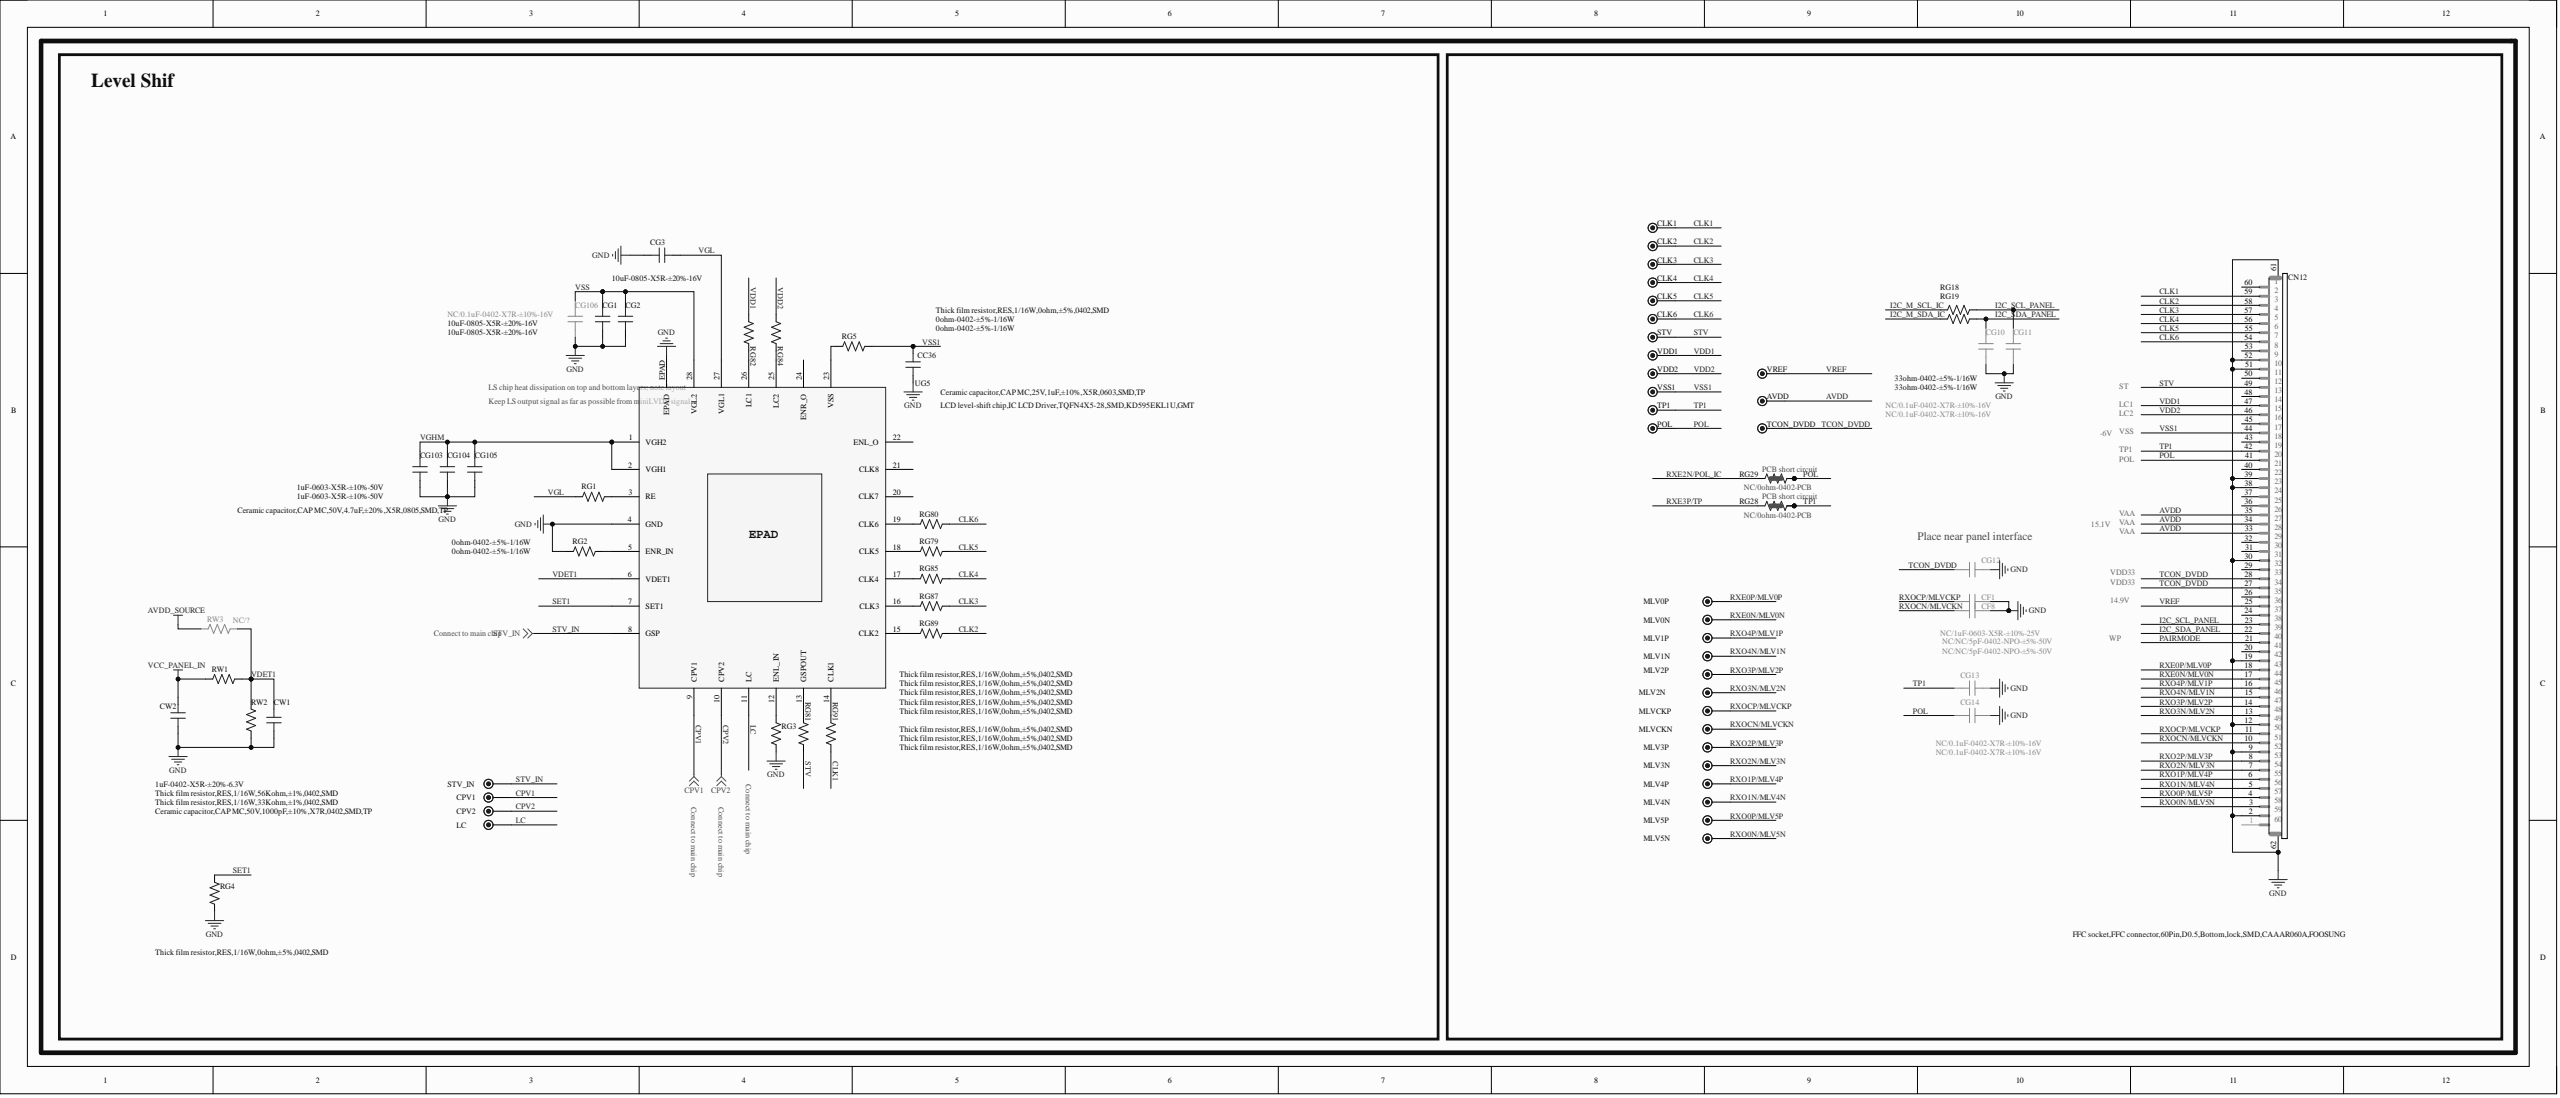Circuit board | Altium Designer | 951 parts | 509 nets | one sheet of the schematic
Parts on this sheet (reference | value | footprint):
CC36 | Ceramic capacitor,CAP MC,25V,1uF,±10%,X5R,0603,SMD,TP | C0603
CF1 | NC/NC/5pF-0402-NPO-±5%-50V | C0402
CF8 | NC/NC/5pF-0402-NPO-±5%-50V | C0402
CG1 | 10uF-0805-X5R-±20%-16V | C0805
CG2 | 10uF-0805-X5R-±20%-16V | C0805
CG3 | 10uF-0805-X5R-±20%-16V | C0805
CG10 | NC/0.1uF-0402-X7R-±10%-16V | C0402
CG11 | NC/0.1uF-0402-X7R-±10%-16V | C0402
CG12 | NC/1uF-0603-X5R-±10%-25V | C0603
CG13 | NC/0.1uF-0402-X7R-±10%-16V | C0402
CG14 | NC/0.1uF-0402-X7R-±10%-16V | C0402
CG103 | 1uF-0603-X5R-±10%-50V | C0603
CG104 | Ceramic capacitor,CAP MC,50V,4.7uF,±20%,X5R,0805,SMD,TP | C0805
CG105 | 1uF-0603-X5R-±10%-50V | C0603
CG106 | NC/0.1uF-0402-X7R-±10%-16V | C0402
CLK1 | TEST | TP
CLK2 | TEST | TP
CLK3 | TEST | TP
CLK4 | TEST | TP
CLK5 | TEST | TP
CLK6 | TEST | TP
CN12 | FFC socket,FFC connector,60Pin,D0.5,Bottom,lock,SMD,CAAAR060A,FOOSUNG | FFC60H/0.5S-13
CW1 | Ceramic capacitor,CAP MC,50V,1000pF,±10%,X7R,0402,SMD,TP | C0402
CW2 | 1uF-0402-X5R-±20%-6.3V | C0402
MLV0N | TEST | TP
MLV0P | TEST | TP
MLV1N | TEST | TP
MLV1P | TEST | TP
MLV2N | TEST | TP
MLV2P | TEST | TP
MLV3N | TEST | TP
MLV3P | TEST | TP
MLV4N | TEST | TP
MLV4P | TEST | TP
MLV5N | TEST | TP
MLV5P | TEST | TP
MLVCKN | TEST | TP
MLVCKP | TEST | TP
POL | TEST | TP
RG1 | 0ohm-0402-±5%-1/16W | R0402
RG2 | 0ohm-0402-±5%-1/16W | R0402
RG4 | Thick film resistor,RES,1/16W,0ohm,±5%,0402,SMD | R0402
RG5 | 0ohm-0402-±5%-1/16W | R0402
RG18 | 33ohm-0402-±5%-1/16W | R0402
RG19 | 33ohm-0402-±5%-1/16W | R0402
RG28 | NC/0ohm-0402-PCB | R0402SC
RG29 | NC/0ohm-0402-PCB | R0402SC
RG79 | Thick film resistor,RES,1/16W,0ohm,±5%,0402,SMD | R0402
RG80 | Thick film resistor,RES,1/16W,0ohm,±5%,0402,SMD | R0402
RG81 | Thick film resistor,RES,1/16W,0ohm,±5%,0402,SMD | R0402
RG82 | Thick film resistor,RES,1/16W,0ohm,±5%,0402,SMD | R0402
RG84 | 0ohm-0402-±5%-1/16W | R0402
RG85 | Thick film resistor,RES,1/16W,0ohm,±5%,0402,SMD | R0402
RG87 | Thick film resistor,RES,1/16W,0ohm,±5%,0402,SMD | R0402
RG89 | Thick film resistor,RES,1/16W,0ohm,±5%,0402,SMD | R0402
RG91 | Thick film resistor,RES,1/16W,0ohm,±5%,0402,SMD | R0402
RW1 | Thick film resistor,RES,1/16W,56Kohm,±1%,0402,SMD | R0402
RW2 | Thick film resistor,RES,1/16W,33Kohm,±1%,0402,SMD | R0402
RW3 | NC/? | R0402
STV | TEST | TP
TP1 | TEST | TP
UG5 | LCD level-shift chip,IC LCD Driver,TQFN4X5-28,SMD,KD595EKL1U,GMT | QFN28/0.5-5
VDD1 | TEST | TP
VDD2 | TEST | TP
VSS1 | TEST | TP
Nets of these parts (net: part-pin ...):
VSS1: CC36-1 RG5-1 VSS1-1 CN12-44
VSS: CG1-1 CG2-1 CG106-2 UG5-28
VREF: CN12-25
VGL: CG3-1 RG1-1 UG5-27
VGHM: CG103-2 CG104-1 CG105-2 UG5-1 UG5-2
VDET1: CW1-2 RW1-2 RW2-2 RW3-2 UG5-6
VDD2: RG84-1 VDD2-1 CN12-46
VDD1: RG82-1 VDD1-1 CN12-47
VCC_PANEL_IN: CW2-1 RW1-1
TP1: CG13-2 RG28-2 RG28-3 TP1-1 CN12-42
TCON_DVDD: CG12-2 CN12-27 CN12-28
STV_IN: UG5-8
STV: RG81-1 STV-1 CN12-49
SET1: RG4-2 UG5-7
RXOCP/MLVCKP: CF1-2 MLVCKP-1 CN12-11
RXOCN/MLVCKN: CF8-2 MLVCKN-1 CN12-10
RXO4P/MLV1P: MLV1P-1 CN12-16
RXO4N/MLV1N: MLV1N-1 CN12-15
RXO3P/MLV2P: MLV2P-1 CN12-14
RXO3N/MLV2N: MLV2N-1 CN12-13
RXO2P/MLV3P: MLV3P-1 CN12-8
RXO2N/MLV3N: MLV3N-1 CN12-7
RXO1P/MLV4P: MLV4P-1 CN12-6
RXO1N/MLV4N: MLV4N-1 CN12-5
RXO0P/MLV5P: MLV5P-1 CN12-4
RXO0N/MLV5N: MLV5N-1 CN12-3
RXE3P/TP: RG28-1
RXE2N/POL_IC: RG29-1
RXE0P/MLV0P: MLV0P-1 CN12-18
RXE0N/MLV0N: MLV0N-1 CN12-17
POL: CG14-2 POL-1 RG29-2 RG29-3 CN12-41
PAIRMODE: CN12-21
NetRG91_1: RG91-1 UG5-14
NetRG89_1: RG89-1 UG5-15
NetRG87_1: RG87-1 UG5-16
NetRG85_1: RG85-1 UG5-17
NetRG84_2: RG84-2 UG5-25
NetRG82_2: RG82-2 UG5-26
NetRG81_2: RG81-2 UG5-13
NetRG80_2: RG80-2 UG5-19
NetRG79_2: RG79-2 UG5-18
NetRG5_2: RG5-2 UG5-23
NetRG2_2: RG2-2 UG5-5
NetRG1_2: RG1-2 UG5-3
LC: UG5-11
I2C_SDA_PANEL: CG10-2 RG19-2 CN12-22
I2C_SCL_PANEL: CG11-2 RG18-2 CN12-23
I2C_M_SDA_IC: RG19-1
I2C_M_SCL_IC: RG18-1
GND: CC36-2 CF1-1 CF8-1 CG1-2 CG2-2 CG3-2 CG10-1 CG11-1 CG12-1 CG13-1 CG14-1 CG103-1 CG104-2 CG105-1 CG106-1 CW1-1 CW2-2 RG2-1 RG4-1 RW2-1 CN12-2 CN12-9 CN12-12 CN12-19 CN12-30 CN12-38 CN12-39 CN12-51 CN12-52 CN12-61 CN12-62 UG5-4 UG5-EPAD
CPV2: UG5-10
CPV1: UG5-9
CLK6: CLK6-1 RG80-1 CN12-54
CLK5: CLK5-1 RG79-1 CN12-55
CLK4: CLK4-1 RG85-2 CN12-56
CLK3: CLK3-1 RG87-2 CN12-57
CLK2: CLK2-1 RG89-2 CN12-58
CLK1: CLK1-1 RG91-2 CN12-59
AVDD_SOURCE: RW3-1
AVDD: CN12-33 CN12-34 CN12-35